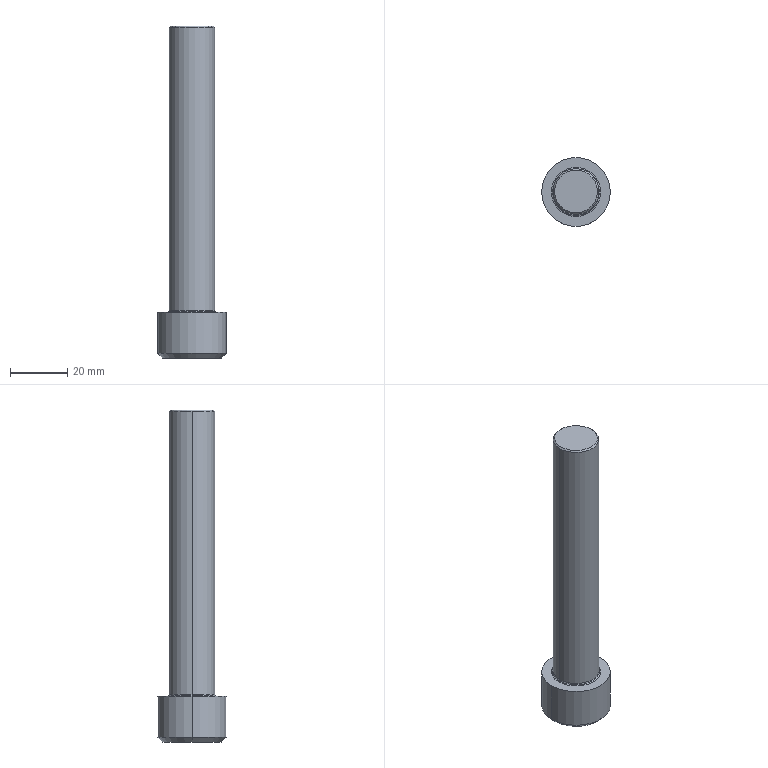Part | Creo | 1 solid | 23 faces | box 24 x 24 x 116 mm | volume 25582 mm3 | plane 9 | cone 6 | cylinder 4 | torus 4 | commonest cylinder face diameters 16 x2 24 x2
STEP:
#1=CARTESIAN_POINT('',(0.,0.,0.));
#2=DIRECTION('',(0.,0.,1.));
#3=DIRECTION('',(1.,0.,0.));
#4=AXIS2_PLACEMENT_3D('',#1,#2,#3);
#5=CARTESIAN_POINT('',(-133.083,-157.,29.5));
#6=VERTEX_POINT('',#5);
#7=CARTESIAN_POINT('',(-129.041,-150.,29.5));
#8=VERTEX_POINT('',#7);
#9=CARTESIAN_POINT('',(-133.083,-157.,29.5));
#10=CARTESIAN_POINT('',(-132.863,-156.619,29.627));
#11=CARTESIAN_POINT('',(-132.422,-155.855,29.851));
#12=CARTESIAN_POINT('',(-131.746,-154.685,30.073));
#13=CARTESIAN_POINT('',(-131.064,-153.504,30.151));
#14=CARTESIAN_POINT('',(-130.379,-152.317,30.073));
#15=CARTESIAN_POINT('',(-129.705,-151.15,29.852));
#16=CARTESIAN_POINT('',(-129.262,-150.382,29.627));
#17=CARTESIAN_POINT('',(-129.041,-150.,29.5));
#18=B_SPLINE_CURVE_WITH_KNOTS('',3,(#9,#10,#11,#12,#13,#14,#15,#16,#17),.UNSPECIFIED.,.F.,.F.,(4,1,1,1,1,1,4),(0.,0.1667,0.3333,0.5,0.6667,0.8333,1.),.UNSPECIFIED.);
#19=EDGE_CURVE('',#6,#8,#18,.T.);
#20=ORIENTED_EDGE('',*,*,#19,.F.);
#21=CARTESIAN_POINT('',(-125.,-157.,34.167));
#22=VERTEX_POINT('',#21);
#23=CARTESIAN_POINT('',(-125.,-157.,34.167));
#24=DIRECTION('',(-0.866,0.,-0.5));
#25=VECTOR('',#24,9.333);
#26=LINE('',#23,#25);
#27=EDGE_CURVE('',#22,#6,#26,.T.);
#28=ORIENTED_EDGE('',*,*,#27,.F.);
#29=CARTESIAN_POINT('',(-116.917,-157.,29.5));
#30=VERTEX_POINT('',#29);
#31=CARTESIAN_POINT('',(-125.,-157.,34.167));
#32=DIRECTION('',(0.866,0.,-0.5));
#33=VECTOR('',#32,9.333);
#34=LINE('',#31,#33);
#35=EDGE_CURVE('',#22,#30,#34,.T.);
#36=ORIENTED_EDGE('',*,*,#35,.T.);
#37=CARTESIAN_POINT('',(-120.959,-150.,29.5));
#38=VERTEX_POINT('',#37);
#39=CARTESIAN_POINT('',(-120.959,-150.,29.5));
#40=CARTESIAN_POINT('',(-120.739,-150.381,29.627));
#41=CARTESIAN_POINT('',(-120.297,-151.145,29.851));
#42=CARTESIAN_POINT('',(-119.622,-152.315,30.073));
#43=CARTESIAN_POINT('',(-118.94,-153.496,30.151));
#44=CARTESIAN_POINT('',(-118.255,-154.683,30.073));
#45=CARTESIAN_POINT('',(-117.581,-155.85,29.852));
#46=CARTESIAN_POINT('',(-117.138,-156.618,29.627));
#47=CARTESIAN_POINT('',(-116.917,-157.,29.5));
#48=B_SPLINE_CURVE_WITH_KNOTS('',3,(#39,#40,#41,#42,#43,#44,#45,#46,#47),.UNSPECIFIED.,.F.,.F.,(4,1,1,1,1,1,4),(0.,0.1667,0.3333,0.5,0.6667,0.8333,1.),.UNSPECIFIED.);
#49=EDGE_CURVE('',#38,#30,#48,.T.);
#50=ORIENTED_EDGE('',*,*,#49,.F.);
#51=CARTESIAN_POINT('',(-129.041,-150.,29.5));
#52=CARTESIAN_POINT('',(-128.604,-150.,29.626));
#53=CARTESIAN_POINT('',(-127.723,-150.,29.85));
#54=CARTESIAN_POINT('',(-126.369,-150.,30.073));
#55=CARTESIAN_POINT('',(-125.002,-150.,30.151));
#56=CARTESIAN_POINT('',(-123.637,-150.,30.074));
#57=CARTESIAN_POINT('',(-122.283,-150.,29.851));
#58=CARTESIAN_POINT('',(-121.399,-150.,29.627));
#59=CARTESIAN_POINT('',(-120.959,-150.,29.5));
#60=B_SPLINE_CURVE_WITH_KNOTS('',3,(#51,#52,#53,#54,#55,#56,#57,#58,#59),.UNSPECIFIED.,.F.,.F.,(4,1,1,1,1,1,4),(0.,0.1667,0.3333,0.5,0.6667,0.8333,1.),.UNSPECIFIED.);
#61=EDGE_CURVE('',#8,#38,#60,.T.);
#62=ORIENTED_EDGE('',*,*,#61,.F.);
#63=EDGE_LOOP('',(#20,#28,#36,#50,#62));
#64=FACE_OUTER_BOUND('',#63,.F.);
#65=CARTESIAN_POINT('',(-125.,-157.,31.787));
#66=DIRECTION('',(0.,0.,-1.));
#67=DIRECTION('',(-1.,0.,0.));
#68=AXIS2_PLACEMENT_3D('',#65,#66,#67);
#69=CONICAL_SURFACE('',#68,4.122,60.);
#70=ADVANCED_FACE('',(#64),#69,.F.);
#71=CARTESIAN_POINT('',(-129.041,-150.,21.5));
#72=VERTEX_POINT('',#71);
#73=CARTESIAN_POINT('',(-133.083,-157.,21.5));
#74=VERTEX_POINT('',#73);
#75=CARTESIAN_POINT('',(-129.041,-150.,21.5));
#76=DIRECTION('',(-0.5,-0.866,0.));
#77=VECTOR('',#76,8.083);
#78=LINE('',#75,#77);
#79=EDGE_CURVE('',#72,#74,#78,.T.);
#80=ORIENTED_EDGE('',*,*,#79,.T.);
#81=CARTESIAN_POINT('',(-133.083,-157.,21.5));
#82=DIRECTION('',(0.,0.,1.));
#83=VECTOR('',#82,8.);
#84=LINE('',#81,#83);
#85=EDGE_CURVE('',#74,#6,#84,.T.);
#86=ORIENTED_EDGE('',*,*,#85,.T.);
#87=ORIENTED_EDGE('',*,*,#19,.T.);
#88=CARTESIAN_POINT('',(-129.041,-150.,21.5));
#89=DIRECTION('',(0.,0.,1.));
#90=VECTOR('',#89,8.);
#91=LINE('',#88,#90);
#92=EDGE_CURVE('',#72,#8,#91,.T.);
#93=ORIENTED_EDGE('',*,*,#92,.F.);
#94=EDGE_LOOP('',(#80,#86,#87,#93));
#95=FACE_OUTER_BOUND('',#94,.F.);
#96=CARTESIAN_POINT('',(-129.041,-150.,29.5));
#97=DIRECTION('',(0.866,-0.5,0.));
#98=DIRECTION('',(-0.5,-0.866,0.));
#99=AXIS2_PLACEMENT_3D('',#96,#97,#98);
#100=PLANE('',#99);
#101=ADVANCED_FACE('',(#95),#100,.T.);
#102=CARTESIAN_POINT('',(-135.4,-157.,21.5));
#103=VERTEX_POINT('',#102);
#104=CARTESIAN_POINT('',(-114.6,-157.,21.5));
#105=VERTEX_POINT('',#104);
#106=CARTESIAN_POINT('',(-125.,-157.,21.5));
#107=DIRECTION('',(0.,0.,-1.));
#108=DIRECTION('',(-1.,0.,0.));
#109=AXIS2_PLACEMENT_3D('',#106,#107,#108);
#110=CIRCLE('',#109,10.4);
#111=EDGE_CURVE('',#103,#105,#110,.T.);
#112=ORIENTED_EDGE('',*,*,#111,.F.);
#113=CARTESIAN_POINT('',(-125.,-157.,21.5));
#114=DIRECTION('',(0.,0.,-1.));
#115=DIRECTION('',(1.,0.,0.));
#116=AXIS2_PLACEMENT_3D('',#113,#114,#115);
#117=CIRCLE('',#116,10.4);
#118=EDGE_CURVE('',#105,#103,#117,.T.);
#119=ORIENTED_EDGE('',*,*,#118,.F.);
#120=EDGE_LOOP('',(#112,#119));
#121=FACE_OUTER_BOUND('',#120,.F.);
#122=CARTESIAN_POINT('',(-129.041,-164.,21.5));
#123=VERTEX_POINT('',#122);
#124=CARTESIAN_POINT('',(-133.083,-157.,21.5));
#125=DIRECTION('',(0.5,-0.866,0.));
#126=VECTOR('',#125,8.083);
#127=LINE('',#124,#126);
#128=EDGE_CURVE('',#74,#123,#127,.T.);
#129=ORIENTED_EDGE('',*,*,#128,.F.);
#130=ORIENTED_EDGE('',*,*,#79,.F.);
#131=CARTESIAN_POINT('',(-120.959,-150.,21.5));
#132=VERTEX_POINT('',#131);
#133=CARTESIAN_POINT('',(-129.041,-150.,21.5));
#134=DIRECTION('',(1.,0.,0.));
#135=VECTOR('',#134,8.083);
#136=LINE('',#133,#135);
#137=EDGE_CURVE('',#72,#132,#136,.T.);
#138=ORIENTED_EDGE('',*,*,#137,.T.);
#139=CARTESIAN_POINT('',(-116.917,-157.,21.5));
#140=VERTEX_POINT('',#139);
#141=CARTESIAN_POINT('',(-116.917,-157.,21.5));
#142=DIRECTION('',(-0.5,0.866,0.));
#143=VECTOR('',#142,8.083);
#144=LINE('',#141,#143);
#145=EDGE_CURVE('',#140,#132,#144,.T.);
#146=ORIENTED_EDGE('',*,*,#145,.F.);
#147=CARTESIAN_POINT('',(-120.959,-164.,21.5));
#148=VERTEX_POINT('',#147);
#149=CARTESIAN_POINT('',(-120.959,-164.,21.5));
#150=DIRECTION('',(0.5,0.866,0.));
#151=VECTOR('',#150,8.083);
#152=LINE('',#149,#151);
#153=EDGE_CURVE('',#148,#140,#152,.T.);
#154=ORIENTED_EDGE('',*,*,#153,.F.);
#155=CARTESIAN_POINT('',(-120.959,-164.,21.5));
#156=DIRECTION('',(-1.,0.,0.));
#157=VECTOR('',#156,8.083);
#158=LINE('',#155,#157);
#159=EDGE_CURVE('',#148,#123,#158,.T.);
#160=ORIENTED_EDGE('',*,*,#159,.T.);
#161=EDGE_LOOP('',(#129,#130,#138,#146,#154,#160));
#162=FACE_BOUND('',#161,.F.);
#163=CARTESIAN_POINT('',(-125.,-157.,21.5));
#164=DIRECTION('',(0.,0.,-1.));
#165=DIRECTION('',(-1.,0.,0.));
#166=AXIS2_PLACEMENT_3D('',#163,#164,#165);
#167=PLANE('',#166);
#168=ADVANCED_FACE('',(#121,#162),#167,.T.);
#169=CARTESIAN_POINT('',(-137.,-157.,23.1));
#170=VERTEX_POINT('',#169);
#171=CARTESIAN_POINT('',(-113.,-157.,23.1));
#172=VERTEX_POINT('',#171);
#173=CARTESIAN_POINT('',(-125.,-157.,23.1));
#174=DIRECTION('',(0.,0.,-1.));
#175=DIRECTION('',(-1.,0.,0.));
#176=AXIS2_PLACEMENT_3D('',#173,#174,#175);
#177=CIRCLE('',#176,12.);
#178=EDGE_CURVE('',#170,#172,#177,.T.);
#179=ORIENTED_EDGE('',*,*,#178,.F.);
#180=CARTESIAN_POINT('',(-135.4,-157.,21.5));
#181=DIRECTION('',(-0.7071,0.,0.7071));
#182=VECTOR('',#181,2.263);
#183=LINE('',#180,#182);
#184=EDGE_CURVE('',#103,#170,#183,.T.);
#185=ORIENTED_EDGE('',*,*,#184,.F.);
#186=ORIENTED_EDGE('',*,*,#111,.T.);
#187=CARTESIAN_POINT('',(-114.6,-157.,21.5));
#188=DIRECTION('',(0.7071,0.,0.7071));
#189=VECTOR('',#188,2.263);
#190=LINE('',#187,#189);
#191=EDGE_CURVE('',#105,#172,#190,.T.);
#192=ORIENTED_EDGE('',*,*,#191,.T.);
#193=EDGE_LOOP('',(#179,#185,#186,#192));
#194=FACE_OUTER_BOUND('',#193,.F.);
#195=CARTESIAN_POINT('',(-125.,-157.,22.3));
#196=DIRECTION('',(0.,0.,1.));
#197=DIRECTION('',(1.,0.,0.));
#198=AXIS2_PLACEMENT_3D('',#195,#196,#197);
#199=CONICAL_SURFACE('',#198,11.2,45.);
#200=ADVANCED_FACE('',(#194),#199,.T.);
#201=ORIENTED_EDGE('',*,*,#178,.T.);
#202=CARTESIAN_POINT('',(-113.,-157.,37.5));
#203=VERTEX_POINT('',#202);
#204=CARTESIAN_POINT('',(-113.,-157.,37.5));
#205=DIRECTION('',(0.,0.,-1.));
#206=VECTOR('',#205,14.4);
#207=LINE('',#204,#206);
#208=EDGE_CURVE('',#203,#172,#207,.T.);
#209=ORIENTED_EDGE('',*,*,#208,.F.);
#210=CARTESIAN_POINT('',(-137.,-157.,37.5));
#211=VERTEX_POINT('',#210);
#212=CARTESIAN_POINT('',(-125.,-157.,37.5));
#213=DIRECTION('',(0.,0.,1.));
#214=DIRECTION('',(1.,0.,0.));
#215=AXIS2_PLACEMENT_3D('',#212,#213,#214);
#216=CIRCLE('',#215,12.);
#217=EDGE_CURVE('',#203,#211,#216,.T.);
#218=ORIENTED_EDGE('',*,*,#217,.T.);
#219=CARTESIAN_POINT('',(-137.,-157.,37.5));
#220=DIRECTION('',(0.,0.,-1.));
#221=VECTOR('',#220,14.4);
#222=LINE('',#219,#221);
#223=EDGE_CURVE('',#211,#170,#222,.T.);
#224=ORIENTED_EDGE('',*,*,#223,.T.);
#225=EDGE_LOOP('',(#201,#209,#218,#224));
#226=FACE_OUTER_BOUND('',#225,.F.);
#227=CARTESIAN_POINT('',(-125.,-157.,37.5));
#228=DIRECTION('',(0.,0.,-1.));
#229=DIRECTION('',(-1.,0.,0.));
#230=AXIS2_PLACEMENT_3D('',#227,#228,#229);
#231=CYLINDRICAL_SURFACE('',#230,12.);
#232=ADVANCED_FACE('',(#226),#231,.T.);
#233=CARTESIAN_POINT('',(-125.,-157.,23.1));
#234=DIRECTION('',(0.,0.,-1.));
#235=DIRECTION('',(1.,0.,0.));
#236=AXIS2_PLACEMENT_3D('',#233,#234,#235);
#237=CIRCLE('',#236,12.);
#238=EDGE_CURVE('',#172,#170,#237,.T.);
#239=ORIENTED_EDGE('',*,*,#238,.T.);
#240=ORIENTED_EDGE('',*,*,#223,.F.);
#241=CARTESIAN_POINT('',(-125.,-157.,37.5));
#242=DIRECTION('',(0.,0.,1.));
#243=DIRECTION('',(-1.,0.,0.));
#244=AXIS2_PLACEMENT_3D('',#241,#242,#243);
#245=CIRCLE('',#244,12.);
#246=EDGE_CURVE('',#211,#203,#245,.T.);
#247=ORIENTED_EDGE('',*,*,#246,.T.);
#248=ORIENTED_EDGE('',*,*,#208,.T.);
#249=EDGE_LOOP('',(#239,#240,#247,#248));
#250=FACE_OUTER_BOUND('',#249,.F.);
#251=CARTESIAN_POINT('',(-125.,-157.,37.5));
#252=DIRECTION('',(0.,0.,-1.));
#253=DIRECTION('',(-1.,0.,0.));
#254=AXIS2_PLACEMENT_3D('',#251,#252,#253);
#255=CYLINDRICAL_SURFACE('',#254,12.);
#256=ADVANCED_FACE('',(#250),#255,.T.);
#257=ORIENTED_EDGE('',*,*,#238,.F.);
#258=ORIENTED_EDGE('',*,*,#191,.F.);
#259=ORIENTED_EDGE('',*,*,#118,.T.);
#260=ORIENTED_EDGE('',*,*,#184,.T.);
#261=EDGE_LOOP('',(#257,#258,#259,#260));
#262=FACE_OUTER_BOUND('',#261,.F.);
#263=CARTESIAN_POINT('',(-125.,-157.,22.3));
#264=DIRECTION('',(0.,0.,1.));
#265=DIRECTION('',(1.,0.,0.));
#266=AXIS2_PLACEMENT_3D('',#263,#264,#265);
#267=CONICAL_SURFACE('',#266,11.2,45.);
#268=ADVANCED_FACE('',(#262),#267,.T.);
#269=ORIENTED_EDGE('',*,*,#246,.F.);
#270=ORIENTED_EDGE('',*,*,#217,.F.);
#271=EDGE_LOOP('',(#269,#270));
#272=FACE_OUTER_BOUND('',#271,.F.);
#273=CARTESIAN_POINT('',(-133.6,-157.,37.5));
#274=VERTEX_POINT('',#273);
#275=CARTESIAN_POINT('',(-116.4,-157.,37.5));
#276=VERTEX_POINT('',#275);
#277=CARTESIAN_POINT('',(-125.,-157.,37.5));
#278=DIRECTION('',(0.,0.,-1.));
#279=DIRECTION('',(-1.,0.,0.));
#280=AXIS2_PLACEMENT_3D('',#277,#278,#279);
#281=CIRCLE('',#280,8.6);
#282=EDGE_CURVE('',#274,#276,#281,.T.);
#283=ORIENTED_EDGE('',*,*,#282,.F.);
#284=CARTESIAN_POINT('',(-125.,-157.,37.5));
#285=DIRECTION('',(0.,0.,-1.));
#286=DIRECTION('',(1.,0.,0.));
#287=AXIS2_PLACEMENT_3D('',#284,#285,#286);
#288=CIRCLE('',#287,8.6);
#289=EDGE_CURVE('',#276,#274,#288,.T.);
#290=ORIENTED_EDGE('',*,*,#289,.F.);
#291=EDGE_LOOP('',(#283,#290));
#292=FACE_BOUND('',#291,.F.);
#293=CARTESIAN_POINT('',(-125.,-157.,37.5));
#294=DIRECTION('',(0.,0.,-1.));
#295=DIRECTION('',(-1.,0.,0.));
#296=AXIS2_PLACEMENT_3D('',#293,#294,#295);
#297=PLANE('',#296);
#298=ADVANCED_FACE('',(#272,#292),#297,.F.);
#299=ORIENTED_EDGE('',*,*,#282,.T.);
#300=CARTESIAN_POINT('',(-116.824,-157.,37.676));
#301=VERTEX_POINT('',#300);
#302=CARTESIAN_POINT('',(-116.4,-157.,38.1));
#303=DIRECTION('',(0.,1.,0.));
#304=DIRECTION('',(0.,0.,-1.));
#305=AXIS2_PLACEMENT_3D('',#302,#303,#304);
#306=CIRCLE('',#305,0.6);
#307=EDGE_CURVE('',#276,#301,#306,.T.);
#308=ORIENTED_EDGE('',*,*,#307,.T.);
#309=CARTESIAN_POINT('',(-133.176,-157.,37.676));
#310=VERTEX_POINT('',#309);
#311=CARTESIAN_POINT('',(-125.,-157.,37.676));
#312=DIRECTION('',(0.,0.,-1.));
#313=DIRECTION('',(-1.,0.,0.));
#314=AXIS2_PLACEMENT_3D('',#311,#312,#313);
#315=CIRCLE('',#314,8.176);
#316=EDGE_CURVE('',#310,#301,#315,.T.);
#317=ORIENTED_EDGE('',*,*,#316,.F.);
#318=CARTESIAN_POINT('',(-133.6,-157.,38.1));
#319=DIRECTION('',(0.,-1.,0.));
#320=DIRECTION('',(0.,0.,-1.));
#321=AXIS2_PLACEMENT_3D('',#318,#319,#320);
#322=CIRCLE('',#321,0.6);
#323=EDGE_CURVE('',#274,#310,#322,.T.);
#324=ORIENTED_EDGE('',*,*,#323,.F.);
#325=EDGE_LOOP('',(#299,#308,#317,#324));
#326=FACE_OUTER_BOUND('',#325,.F.);
#327=CARTESIAN_POINT('',(-125.,-157.,38.1));
#328=DIRECTION('',(0.,0.,-1.));
#329=DIRECTION('',(-1.,0.,0.));
#330=AXIS2_PLACEMENT_3D('',#327,#328,#329);
#331=TOROIDAL_SURFACE('',#330,8.6,0.6);
#332=ADVANCED_FACE('',(#326),#331,.F.);
#333=ORIENTED_EDGE('',*,*,#289,.T.);
#334=ORIENTED_EDGE('',*,*,#323,.T.);
#335=CARTESIAN_POINT('',(-125.,-157.,37.676));
#336=DIRECTION('',(0.,0.,-1.));
#337=DIRECTION('',(1.,0.,0.));
#338=AXIS2_PLACEMENT_3D('',#335,#336,#337);
#339=CIRCLE('',#338,8.176);
#340=EDGE_CURVE('',#301,#310,#339,.T.);
#341=ORIENTED_EDGE('',*,*,#340,.F.);
#342=ORIENTED_EDGE('',*,*,#307,.F.);
#343=EDGE_LOOP('',(#333,#334,#341,#342));
#344=FACE_OUTER_BOUND('',#343,.F.);
#345=CARTESIAN_POINT('',(-125.,-157.,38.1));
#346=DIRECTION('',(0.,0.,-1.));
#347=DIRECTION('',(-1.,0.,0.));
#348=AXIS2_PLACEMENT_3D('',#345,#346,#347);
#349=TOROIDAL_SURFACE('',#348,8.6,0.6);
#350=ADVANCED_FACE('',(#344),#349,.F.);
#351=CARTESIAN_POINT('',(-117.,-157.,38.1));
#352=VERTEX_POINT('',#351);
#353=CARTESIAN_POINT('',(-133.,-157.,38.1));
#354=VERTEX_POINT('',#353);
#355=CARTESIAN_POINT('',(-125.,-157.,38.1));
#356=DIRECTION('',(0.,0.,-1.));
#357=DIRECTION('',(1.,0.,0.));
#358=AXIS2_PLACEMENT_3D('',#355,#356,#357);
#359=CIRCLE('',#358,8.);
#360=EDGE_CURVE('',#352,#354,#359,.T.);
#361=ORIENTED_EDGE('',*,*,#360,.F.);
#362=CARTESIAN_POINT('',(-116.4,-157.,38.1));
#363=DIRECTION('',(0.,1.,0.));
#364=DIRECTION('',(-0.7071,0.,-0.7071));
#365=AXIS2_PLACEMENT_3D('',#362,#363,#364);
#366=CIRCLE('',#365,0.6);
#367=EDGE_CURVE('',#301,#352,#366,.T.);
#368=ORIENTED_EDGE('',*,*,#367,.F.);
#369=ORIENTED_EDGE('',*,*,#340,.T.);
#370=CARTESIAN_POINT('',(-133.6,-157.,38.1));
#371=DIRECTION('',(0.,-1.,0.));
#372=DIRECTION('',(0.7071,0.,-0.7071));
#373=AXIS2_PLACEMENT_3D('',#370,#371,#372);
#374=CIRCLE('',#373,0.6);
#375=EDGE_CURVE('',#310,#354,#374,.T.);
#376=ORIENTED_EDGE('',*,*,#375,.T.);
#377=EDGE_LOOP('',(#361,#368,#369,#376));
#378=FACE_OUTER_BOUND('',#377,.F.);
#379=CARTESIAN_POINT('',(-125.,-157.,38.1));
#380=DIRECTION('',(0.,0.,-1.));
#381=DIRECTION('',(-1.,0.,0.));
#382=AXIS2_PLACEMENT_3D('',#379,#380,#381);
#383=TOROIDAL_SURFACE('',#382,8.6,0.6);
#384=ADVANCED_FACE('',(#378),#383,.F.);
#385=CARTESIAN_POINT('',(-133.,-157.,137.));
#386=VERTEX_POINT('',#385);
#387=CARTESIAN_POINT('',(-117.,-157.,137.));
#388=VERTEX_POINT('',#387);
#389=CARTESIAN_POINT('',(-125.,-157.,137.));
#390=DIRECTION('',(0.,0.,1.));
#391=DIRECTION('',(-1.,0.,0.));
#392=AXIS2_PLACEMENT_3D('',#389,#390,#391);
#393=CIRCLE('',#392,8.);
#394=EDGE_CURVE('',#386,#388,#393,.T.);
#395=ORIENTED_EDGE('',*,*,#394,.T.);
#396=CARTESIAN_POINT('',(-117.,-157.,137.));
#397=DIRECTION('',(0.,0.,-1.));
#398=VECTOR('',#397,98.9);
#399=LINE('',#396,#398);
#400=EDGE_CURVE('',#388,#352,#399,.T.);
#401=ORIENTED_EDGE('',*,*,#400,.T.);
#402=ORIENTED_EDGE('',*,*,#360,.T.);
#403=CARTESIAN_POINT('',(-133.,-157.,137.));
#404=DIRECTION('',(0.,0.,-1.));
#405=VECTOR('',#404,98.9);
#406=LINE('',#403,#405);
#407=EDGE_CURVE('',#386,#354,#406,.T.);
#408=ORIENTED_EDGE('',*,*,#407,.F.);
#409=EDGE_LOOP('',(#395,#401,#402,#408));
#410=FACE_OUTER_BOUND('',#409,.F.);
#411=CARTESIAN_POINT('',(-125.,-157.,137.5));
#412=DIRECTION('',(0.,0.,-1.));
#413=DIRECTION('',(-1.,0.,0.));
#414=AXIS2_PLACEMENT_3D('',#411,#412,#413);
#415=CYLINDRICAL_SURFACE('',#414,8.);
#416=ADVANCED_FACE('',(#410),#415,.T.);
#417=CARTESIAN_POINT('',(-132.5,-157.,137.5));
#418=VERTEX_POINT('',#417);
#419=CARTESIAN_POINT('',(-117.5,-157.,137.5));
#420=VERTEX_POINT('',#419);
#421=CARTESIAN_POINT('',(-125.,-157.,137.5));
#422=DIRECTION('',(0.,0.,1.));
#423=DIRECTION('',(-1.,0.,0.));
#424=AXIS2_PLACEMENT_3D('',#421,#422,#423);
#425=CIRCLE('',#424,7.5);
#426=EDGE_CURVE('',#418,#420,#425,.T.);
#427=ORIENTED_EDGE('',*,*,#426,.T.);
#428=CARTESIAN_POINT('',(-117.5,-157.,137.5));
#429=DIRECTION('',(0.7071,0.,-0.7071));
#430=VECTOR('',#429,0.7071);
#431=LINE('',#428,#430);
#432=EDGE_CURVE('',#420,#388,#431,.T.);
#433=ORIENTED_EDGE('',*,*,#432,.T.);
#434=ORIENTED_EDGE('',*,*,#394,.F.);
#435=CARTESIAN_POINT('',(-132.5,-157.,137.5));
#436=DIRECTION('',(-0.7071,0.,-0.7071));
#437=VECTOR('',#436,0.7071);
#438=LINE('',#435,#437);
#439=EDGE_CURVE('',#418,#386,#438,.T.);
#440=ORIENTED_EDGE('',*,*,#439,.F.);
#441=EDGE_LOOP('',(#427,#433,#434,#440));
#442=FACE_OUTER_BOUND('',#441,.F.);
#443=CARTESIAN_POINT('',(-125.,-157.,137.25));
#444=DIRECTION('',(0.,0.,-1.));
#445=DIRECTION('',(-1.,0.,0.));
#446=AXIS2_PLACEMENT_3D('',#443,#444,#445);
#447=CONICAL_SURFACE('',#446,7.75,45.);
#448=ADVANCED_FACE('',(#442),#447,.T.);
#449=ORIENTED_EDGE('',*,*,#426,.F.);
#450=CARTESIAN_POINT('',(-125.,-157.,137.5));
#451=DIRECTION('',(0.,0.,1.));
#452=DIRECTION('',(1.,0.,0.));
#453=AXIS2_PLACEMENT_3D('',#450,#451,#452);
#454=CIRCLE('',#453,7.5);
#455=EDGE_CURVE('',#420,#418,#454,.T.);
#456=ORIENTED_EDGE('',*,*,#455,.F.);
#457=EDGE_LOOP('',(#449,#456));
#458=FACE_OUTER_BOUND('',#457,.F.);
#459=CARTESIAN_POINT('',(-125.,-157.,137.5));
#460=DIRECTION('',(0.,0.,-1.));
#461=DIRECTION('',(-1.,0.,0.));
#462=AXIS2_PLACEMENT_3D('',#459,#460,#461);
#463=PLANE('',#462);
#464=ADVANCED_FACE('',(#458),#463,.F.);
#465=ORIENTED_EDGE('',*,*,#455,.T.);
#466=ORIENTED_EDGE('',*,*,#439,.T.);
#467=CARTESIAN_POINT('',(-125.,-157.,137.));
#468=DIRECTION('',(0.,0.,1.));
#469=DIRECTION('',(1.,0.,0.));
#470=AXIS2_PLACEMENT_3D('',#467,#468,#469);
#471=CIRCLE('',#470,8.);
#472=EDGE_CURVE('',#388,#386,#471,.T.);
#473=ORIENTED_EDGE('',*,*,#472,.F.);
#474=ORIENTED_EDGE('',*,*,#432,.F.);
#475=EDGE_LOOP('',(#465,#466,#473,#474));
#476=FACE_OUTER_BOUND('',#475,.F.);
#477=CARTESIAN_POINT('',(-125.,-157.,137.25));
#478=DIRECTION('',(0.,0.,-1.));
#479=DIRECTION('',(-1.,0.,0.));
#480=AXIS2_PLACEMENT_3D('',#477,#478,#479);
#481=CONICAL_SURFACE('',#480,7.75,45.);
#482=ADVANCED_FACE('',(#476),#481,.T.);
#483=ORIENTED_EDGE('',*,*,#472,.T.);
#484=ORIENTED_EDGE('',*,*,#407,.T.);
#485=CARTESIAN_POINT('',(-125.,-157.,38.1));
#486=DIRECTION('',(0.,0.,-1.));
#487=DIRECTION('',(-1.,0.,0.));
#488=AXIS2_PLACEMENT_3D('',#485,#486,#487);
#489=CIRCLE('',#488,8.);
#490=EDGE_CURVE('',#354,#352,#489,.T.);
#491=ORIENTED_EDGE('',*,*,#490,.T.);
#492=ORIENTED_EDGE('',*,*,#400,.F.);
#493=EDGE_LOOP('',(#483,#484,#491,#492));
#494=FACE_OUTER_BOUND('',#493,.F.);
#495=CARTESIAN_POINT('',(-125.,-157.,137.5));
#496=DIRECTION('',(0.,0.,-1.));
#497=DIRECTION('',(-1.,0.,0.));
#498=AXIS2_PLACEMENT_3D('',#495,#496,#497);
#499=CYLINDRICAL_SURFACE('',#498,8.);
#500=ADVANCED_FACE('',(#494),#499,.T.);
#501=ORIENTED_EDGE('',*,*,#490,.F.);
#502=ORIENTED_EDGE('',*,*,#375,.F.);
#503=ORIENTED_EDGE('',*,*,#316,.T.);
#504=ORIENTED_EDGE('',*,*,#367,.T.);
#505=EDGE_LOOP('',(#501,#502,#503,#504));
#506=FACE_OUTER_BOUND('',#505,.F.);
#507=CARTESIAN_POINT('',(-125.,-157.,38.1));
#508=DIRECTION('',(0.,0.,-1.));
#509=DIRECTION('',(-1.,0.,0.));
#510=AXIS2_PLACEMENT_3D('',#507,#508,#509);
#511=TOROIDAL_SURFACE('',#510,8.6,0.6);
#512=ADVANCED_FACE('',(#506),#511,.F.);
#513=ORIENTED_EDGE('',*,*,#128,.T.);
#514=CARTESIAN_POINT('',(-129.041,-164.,29.5));
#515=VERTEX_POINT('',#514);
#516=CARTESIAN_POINT('',(-129.041,-164.,21.5));
#517=DIRECTION('',(0.,0.,1.));
#518=VECTOR('',#517,8.);
#519=LINE('',#516,#518);
#520=EDGE_CURVE('',#123,#515,#519,.T.);
#521=ORIENTED_EDGE('',*,*,#520,.T.);
#522=CARTESIAN_POINT('',(-129.041,-164.,29.5));
#523=CARTESIAN_POINT('',(-129.261,-163.619,29.627));
#524=CARTESIAN_POINT('',(-129.703,-162.855,29.851));
#525=CARTESIAN_POINT('',(-130.378,-161.685,30.073));
#526=CARTESIAN_POINT('',(-131.06,-160.504,30.151));
#527=CARTESIAN_POINT('',(-131.745,-159.317,30.073));
#528=CARTESIAN_POINT('',(-132.419,-158.15,29.852));
#529=CARTESIAN_POINT('',(-132.862,-157.382,29.627));
#530=CARTESIAN_POINT('',(-133.083,-157.,29.5));
#531=B_SPLINE_CURVE_WITH_KNOTS('',3,(#522,#523,#524,#525,#526,#527,#528,#529,#530),.UNSPECIFIED.,.F.,.F.,(4,1,1,1,1,1,4),(0.,0.1667,0.3333,0.5,0.6667,0.8333,1.),.UNSPECIFIED.);
#532=EDGE_CURVE('',#515,#6,#531,.T.);
#533=ORIENTED_EDGE('',*,*,#532,.T.);
#534=ORIENTED_EDGE('',*,*,#85,.F.);
#535=EDGE_LOOP('',(#513,#521,#533,#534));
#536=FACE_OUTER_BOUND('',#535,.F.);
#537=CARTESIAN_POINT('',(-133.083,-157.,29.5));
#538=DIRECTION('',(0.866,0.5,0.));
#539=DIRECTION('',(0.5,-0.866,0.));
#540=AXIS2_PLACEMENT_3D('',#537,#538,#539);
#541=PLANE('',#540);
#542=ADVANCED_FACE('',(#536),#541,.T.);
#543=ORIENTED_EDGE('',*,*,#159,.F.);
#544=CARTESIAN_POINT('',(-120.959,-164.,29.5));
#545=VERTEX_POINT('',#544);
#546=CARTESIAN_POINT('',(-120.959,-164.,21.5));
#547=DIRECTION('',(0.,0.,1.));
#548=VECTOR('',#547,8.);
#549=LINE('',#546,#548);
#550=EDGE_CURVE('',#148,#545,#549,.T.);
#551=ORIENTED_EDGE('',*,*,#550,.T.);
#552=CARTESIAN_POINT('',(-120.959,-164.,29.5));
#553=CARTESIAN_POINT('',(-121.399,-164.,29.627));
#554=CARTESIAN_POINT('',(-122.283,-164.,29.851));
#555=CARTESIAN_POINT('',(-123.637,-164.,30.074));
#556=CARTESIAN_POINT('',(-125.002,-164.,30.151));
#557=CARTESIAN_POINT('',(-126.369,-164.,30.073));
#558=CARTESIAN_POINT('',(-127.723,-164.,29.85));
#559=CARTESIAN_POINT('',(-128.604,-164.,29.626));
#560=CARTESIAN_POINT('',(-129.041,-164.,29.5));
#561=B_SPLINE_CURVE_WITH_KNOTS('',3,(#552,#553,#554,#555,#556,#557,#558,#559,#560),.UNSPECIFIED.,.F.,.F.,(4,1,1,1,1,1,4),(0.,0.1667,0.3333,0.5,0.6667,0.8333,1.),.UNSPECIFIED.);
#562=EDGE_CURVE('',#545,#515,#561,.T.);
#563=ORIENTED_EDGE('',*,*,#562,.T.);
#564=ORIENTED_EDGE('',*,*,#520,.F.);
#565=EDGE_LOOP('',(#543,#551,#563,#564));
#566=FACE_OUTER_BOUND('',#565,.F.);
#567=CARTESIAN_POINT('',(-129.041,-164.,29.5));
#568=DIRECTION('',(0.,1.,0.));
#569=DIRECTION('',(0.,0.,-1.));
#570=AXIS2_PLACEMENT_3D('',#567,#568,#569);
#571=PLANE('',#570);
#572=ADVANCED_FACE('',(#566),#571,.T.);
#573=ORIENTED_EDGE('',*,*,#153,.T.);
#574=CARTESIAN_POINT('',(-116.917,-157.,21.5));
#575=DIRECTION('',(0.,0.,1.));
#576=VECTOR('',#575,8.);
#577=LINE('',#574,#576);
#578=EDGE_CURVE('',#140,#30,#577,.T.);
#579=ORIENTED_EDGE('',*,*,#578,.T.);
#580=CARTESIAN_POINT('',(-116.917,-157.,29.5));
#581=CARTESIAN_POINT('',(-117.138,-157.382,29.627));
#582=CARTESIAN_POINT('',(-117.581,-158.15,29.852));
#583=CARTESIAN_POINT('',(-118.255,-159.317,30.073));
#584=CARTESIAN_POINT('',(-118.94,-160.504,30.151));
#585=CARTESIAN_POINT('',(-119.622,-161.685,30.073));
#586=CARTESIAN_POINT('',(-120.297,-162.855,29.851));
#587=CARTESIAN_POINT('',(-120.739,-163.619,29.627));
#588=CARTESIAN_POINT('',(-120.959,-164.,29.5));
#589=B_SPLINE_CURVE_WITH_KNOTS('',3,(#580,#581,#582,#583,#584,#585,#586,#587,#588),.UNSPECIFIED.,.F.,.F.,(4,1,1,1,1,1,4),(0.,0.1667,0.3333,0.5,0.6667,0.8333,1.),.UNSPECIFIED.);
#590=EDGE_CURVE('',#30,#545,#589,.T.);
#591=ORIENTED_EDGE('',*,*,#590,.T.);
#592=ORIENTED_EDGE('',*,*,#550,.F.);
#593=EDGE_LOOP('',(#573,#579,#591,#592));
#594=FACE_OUTER_BOUND('',#593,.F.);
#595=CARTESIAN_POINT('',(-120.959,-164.,29.5));
#596=DIRECTION('',(-0.866,0.5,0.));
#597=DIRECTION('',(0.5,0.866,0.));
#598=AXIS2_PLACEMENT_3D('',#595,#596,#597);
#599=PLANE('',#598);
#600=ADVANCED_FACE('',(#594),#599,.T.);
#601=ORIENTED_EDGE('',*,*,#145,.T.);
#602=CARTESIAN_POINT('',(-120.959,-150.,21.5));
#603=DIRECTION('',(0.,0.,1.));
#604=VECTOR('',#603,8.);
#605=LINE('',#602,#604);
#606=EDGE_CURVE('',#132,#38,#605,.T.);
#607=ORIENTED_EDGE('',*,*,#606,.T.);
#608=ORIENTED_EDGE('',*,*,#49,.T.);
#609=ORIENTED_EDGE('',*,*,#578,.F.);
#610=EDGE_LOOP('',(#601,#607,#608,#609));
#611=FACE_OUTER_BOUND('',#610,.F.);
#612=CARTESIAN_POINT('',(-116.917,-157.,29.5));
#613=DIRECTION('',(-0.866,-0.5,0.));
#614=DIRECTION('',(-0.5,0.866,0.));
#615=AXIS2_PLACEMENT_3D('',#612,#613,#614);
#616=PLANE('',#615);
#617=ADVANCED_FACE('',(#611),#616,.T.);
#618=ORIENTED_EDGE('',*,*,#137,.F.);
#619=ORIENTED_EDGE('',*,*,#92,.T.);
#620=ORIENTED_EDGE('',*,*,#61,.T.);
#621=ORIENTED_EDGE('',*,*,#606,.F.);
#622=EDGE_LOOP('',(#618,#619,#620,#621));
#623=FACE_OUTER_BOUND('',#622,.F.);
#624=CARTESIAN_POINT('',(-120.959,-150.,29.5));
#625=DIRECTION('',(0.,-1.,0.));
#626=DIRECTION('',(0.,0.,1.));
#627=AXIS2_PLACEMENT_3D('',#624,#625,#626);
#628=PLANE('',#627);
#629=ADVANCED_FACE('',(#623),#628,.T.);
#630=ORIENTED_EDGE('',*,*,#590,.F.);
#631=ORIENTED_EDGE('',*,*,#35,.F.);
#632=ORIENTED_EDGE('',*,*,#27,.T.);
#633=ORIENTED_EDGE('',*,*,#532,.F.);
#634=ORIENTED_EDGE('',*,*,#562,.F.);
#635=EDGE_LOOP('',(#630,#631,#632,#633,#634));
#636=FACE_OUTER_BOUND('',#635,.F.);
#637=CARTESIAN_POINT('',(-125.,-157.,31.787));
#638=DIRECTION('',(0.,0.,-1.));
#639=DIRECTION('',(-1.,0.,0.));
#640=AXIS2_PLACEMENT_3D('',#637,#638,#639);
#641=CONICAL_SURFACE('',#640,4.122,60.);
#642=ADVANCED_FACE('',(#636),#641,.F.);
#643=CLOSED_SHELL('',(#70,#101,#168,#200,#232,#256,#268,#298,#332,#350,#384,#416,#448,#464,#482,#500,#512,#542,#572,#600,#617,#629,#642));
#644=MANIFOLD_SOLID_BREP('',#643);
#645=(LENGTH_UNIT()NAMED_UNIT(*)SI_UNIT(.MILLI.,.METRE.));
#646=UNCERTAINTY_MEASURE_WITH_UNIT(LENGTH_MEASURE(0.01209),#645,'','');
#647=(NAMED_UNIT(*)PLANE_ANGLE_UNIT()SI_UNIT($,.RADIAN.));
#648=PLANE_ANGLE_MEASURE_WITH_UNIT(PLANE_ANGLE_MEASURE(0.01745),#647);
#649=(CONVERSION_BASED_UNIT('DEGREE',#648)NAMED_UNIT(*)PLANE_ANGLE_UNIT());
#650=(NAMED_UNIT(*)SI_UNIT($,.STERADIAN.)SOLID_ANGLE_UNIT());
#651=(GEOMETRIC_REPRESENTATION_CONTEXT(3)GLOBAL_UNCERTAINTY_ASSIGNED_CONTEXT((#646))GLOBAL_UNIT_ASSIGNED_CONTEXT((#645,#649,#650))REPRESENTATION_CONTEXT('',''));
#652=ADVANCED_BREP_SHAPE_REPRESENTATION('',(#4,#644),#651);